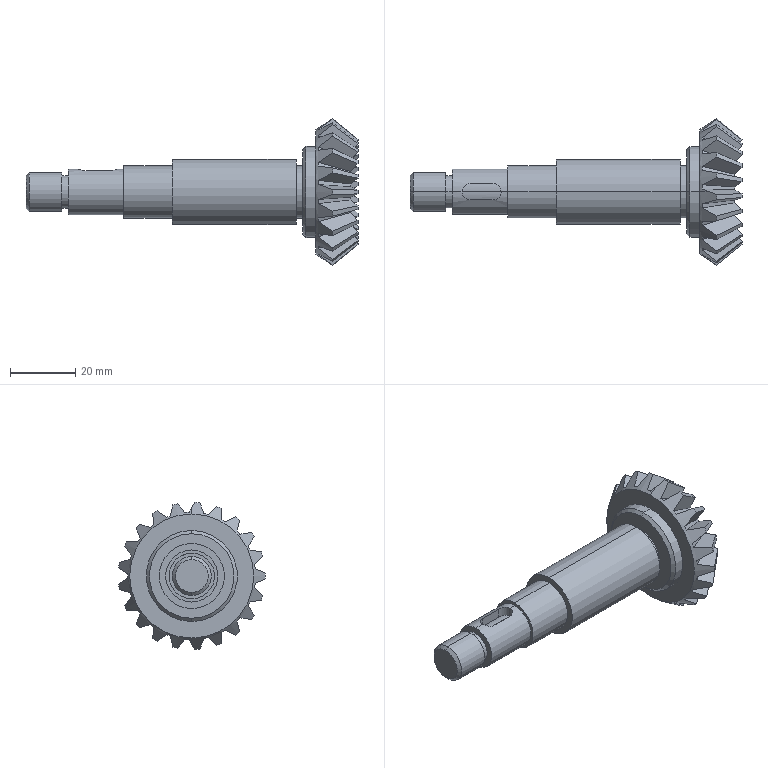Part | SolidWorks | features ICE 7, BlendCut 1, Chamfer 1, CirPattern 1, Extrusion 1, Revolution 1, StudWizard 1 | 1 solid | 121 faces | box 102 x 45.084 x 45.195 mm | volume 33414 mm3 | plane 74 | cone 29 | cylinder 16 | spline 2 | commonest cylinder face diameters 14 x4 16 x4 10 x2 12 x2 20 x2 28 x2